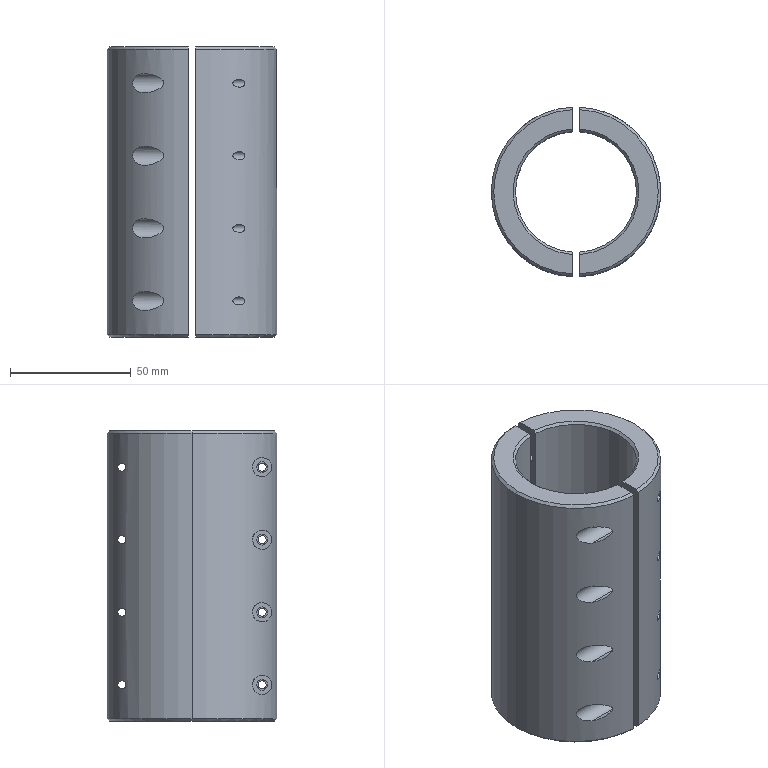Part | SolidWorks | features BaseBody 2 | 2 solids | 82 faces | box 70 x 69.936 x 120 mm | volume 211353 mm3 | cylinder 54 | plane 16 | cone 12 | commonest cylinder face diameters 3.3 x16 4.5 x16 8 x16 50 x3 70 x3